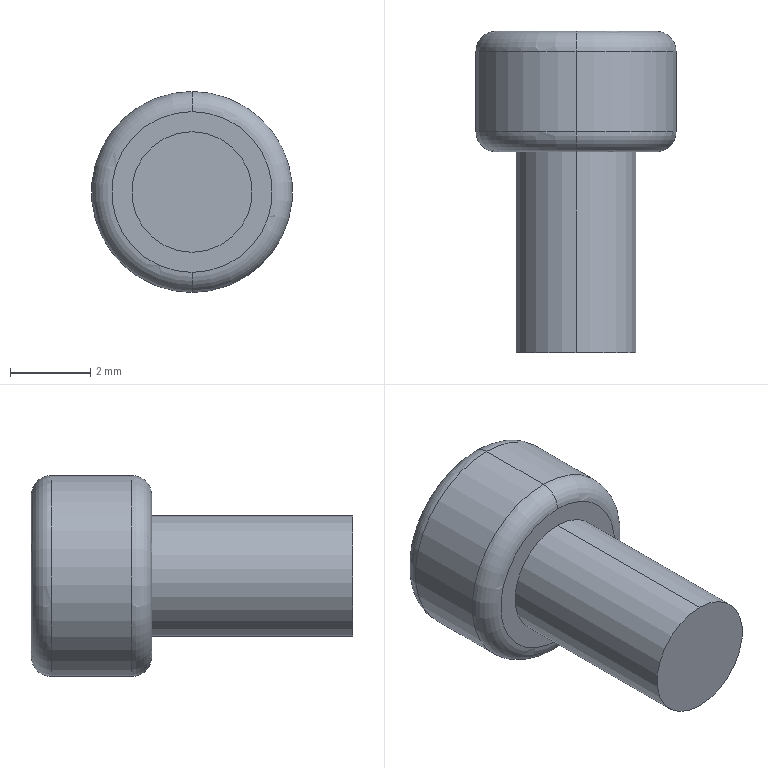Part | NX | features BREP 1 | 1 solid | 18 faces | box 5 x 8 x 5 mm | volume 87.225 mm3 | plane 10 | torus 4 | cylinder 4 | commonest cylinder face diameters 3 x2 5 x2
STEP:
#1=CARTESIAN_POINT('',(0.,2.5,-2.5));
#2=VERTEX_POINT('',#1);
#3=CARTESIAN_POINT('',(0.,2.5,2.5));
#4=VERTEX_POINT('',#3);
#5=CARTESIAN_POINT('',(0.,2.5,0.));
#6=DIRECTION('',(0.,-1.,0.));
#7=DIRECTION('',(0.,0.,1.));
#8=AXIS2_PLACEMENT_3D('',#5,#6,#7);
#9=CIRCLE('',#8,2.5);
#10=EDGE_CURVE('',#2,#4,#9,.T.);
#11=ORIENTED_EDGE('',*,*,#10,.F.);
#12=CARTESIAN_POINT('',(0.,3.,-2.));
#13=VERTEX_POINT('',#12);
#14=CARTESIAN_POINT('',(0.,2.5,-2.));
#15=DIRECTION('',(1.,0.,0.));
#16=DIRECTION('',(0.,0.,-1.));
#17=AXIS2_PLACEMENT_3D('',#14,#15,#16);
#18=CIRCLE('',#17,0.5);
#19=EDGE_CURVE('',#2,#13,#18,.T.);
#20=ORIENTED_EDGE('',*,*,#19,.T.);
#21=CARTESIAN_POINT('',(0.,3.,2.));
#22=VERTEX_POINT('',#21);
#23=CARTESIAN_POINT('',(0.,3.,0.));
#24=DIRECTION('',(0.,1.,0.));
#25=DIRECTION('',(0.,0.,1.));
#26=AXIS2_PLACEMENT_3D('',#23,#24,#25);
#27=CIRCLE('',#26,2.);
#28=EDGE_CURVE('',#22,#13,#27,.T.);
#29=ORIENTED_EDGE('',*,*,#28,.F.);
#30=CARTESIAN_POINT('',(0.,2.5,2.));
#31=DIRECTION('',(-1.,0.,0.));
#32=DIRECTION('',(0.,0.,1.));
#33=AXIS2_PLACEMENT_3D('',#30,#31,#32);
#34=CIRCLE('',#33,0.5);
#35=EDGE_CURVE('',#4,#22,#34,.T.);
#36=ORIENTED_EDGE('',*,*,#35,.F.);
#37=EDGE_LOOP('',(#11,#20,#29,#36));
#38=FACE_BOUND('',#37,.T.);
#39=CARTESIAN_POINT('',(0.,2.5,0.));
#40=DIRECTION('',(0.,1.,0.));
#41=DIRECTION('',(0.,0.,-1.));
#42=AXIS2_PLACEMENT_3D('',#39,#40,#41);
#43=TOROIDAL_SURFACE('',#42,2.,0.5);
#44=ADVANCED_FACE('',(#38),#43,.T.);
#45=CARTESIAN_POINT('',(0.,0.,-2.));
#46=VERTEX_POINT('',#45);
#47=CARTESIAN_POINT('',(0.,0.,2.));
#48=VERTEX_POINT('',#47);
#49=CARTESIAN_POINT('',(0.,0.,0.));
#50=DIRECTION('',(0.,-1.,0.));
#51=DIRECTION('',(0.,0.,1.));
#52=AXIS2_PLACEMENT_3D('',#49,#50,#51);
#53=CIRCLE('',#52,2.);
#54=EDGE_CURVE('',#46,#48,#53,.T.);
#55=ORIENTED_EDGE('',*,*,#54,.F.);
#56=CARTESIAN_POINT('',(0.,0.5,-2.5));
#57=VERTEX_POINT('',#56);
#58=CARTESIAN_POINT('',(0.,0.5,-2.));
#59=DIRECTION('',(1.,0.,0.));
#60=DIRECTION('',(0.,0.,-1.));
#61=AXIS2_PLACEMENT_3D('',#58,#59,#60);
#62=CIRCLE('',#61,0.5);
#63=EDGE_CURVE('',#46,#57,#62,.T.);
#64=ORIENTED_EDGE('',*,*,#63,.T.);
#65=CARTESIAN_POINT('',(0.,0.5,2.5));
#66=VERTEX_POINT('',#65);
#67=CARTESIAN_POINT('',(0.,0.5,0.));
#68=DIRECTION('',(0.,1.,0.));
#69=DIRECTION('',(0.,0.,1.));
#70=AXIS2_PLACEMENT_3D('',#67,#68,#69);
#71=CIRCLE('',#70,2.5);
#72=EDGE_CURVE('',#66,#57,#71,.T.);
#73=ORIENTED_EDGE('',*,*,#72,.F.);
#74=CARTESIAN_POINT('',(0.,0.5,2.));
#75=DIRECTION('',(-1.,0.,0.));
#76=DIRECTION('',(0.,0.,1.));
#77=AXIS2_PLACEMENT_3D('',#74,#75,#76);
#78=CIRCLE('',#77,0.5);
#79=EDGE_CURVE('',#48,#66,#78,.T.);
#80=ORIENTED_EDGE('',*,*,#79,.F.);
#81=EDGE_LOOP('',(#55,#64,#73,#80));
#82=FACE_BOUND('',#81,.T.);
#83=CARTESIAN_POINT('',(0.,0.5,0.));
#84=DIRECTION('',(0.,1.,0.));
#85=DIRECTION('',(0.,0.,-1.));
#86=AXIS2_PLACEMENT_3D('',#83,#84,#85);
#87=TOROIDAL_SURFACE('',#86,2.,0.5);
#88=ADVANCED_FACE('',(#82),#87,.T.);
#89=CARTESIAN_POINT('',(0.,-5.,-1.5));
#90=VERTEX_POINT('',#89);
#91=CARTESIAN_POINT('',(0.,-5.,1.5));
#92=VERTEX_POINT('',#91);
#93=CARTESIAN_POINT('',(0.,-5.,0.));
#94=DIRECTION('',(0.,-1.,0.));
#95=DIRECTION('',(0.,0.,-1.));
#96=AXIS2_PLACEMENT_3D('',#93,#94,#95);
#97=CIRCLE('',#96,1.5);
#98=EDGE_CURVE('',#90,#92,#97,.T.);
#99=ORIENTED_EDGE('',*,*,#98,.F.);
#100=CARTESIAN_POINT('',(0.,0.,-1.5));
#101=VERTEX_POINT('',#100);
#102=CARTESIAN_POINT('',(0.,-5.,-1.5));
#103=DIRECTION('',(0.,1.,0.));
#104=VECTOR('',#103,1000.);
#105=LINE('',#102,#104);
#106=EDGE_CURVE('',#90,#101,#105,.T.);
#107=ORIENTED_EDGE('',*,*,#106,.T.);
#108=CARTESIAN_POINT('',(0.,0.,1.5));
#109=VERTEX_POINT('',#108);
#110=CARTESIAN_POINT('',(0.,0.,0.));
#111=DIRECTION('',(0.,-1.,0.));
#112=DIRECTION('',(0.,0.,-1.));
#113=AXIS2_PLACEMENT_3D('',#110,#111,#112);
#114=CIRCLE('',#113,1.5);
#115=EDGE_CURVE('',#101,#109,#114,.T.);
#116=ORIENTED_EDGE('',*,*,#115,.T.);
#117=CARTESIAN_POINT('',(0.,-5.,1.5));
#118=DIRECTION('',(0.,1.,0.));
#119=VECTOR('',#118,1000.);
#120=LINE('',#117,#119);
#121=EDGE_CURVE('',#92,#109,#120,.T.);
#122=ORIENTED_EDGE('',*,*,#121,.F.);
#123=EDGE_LOOP('',(#99,#107,#116,#122));
#124=FACE_BOUND('',#123,.T.);
#125=CARTESIAN_POINT('',(0.,-5.,0.));
#126=DIRECTION('',(0.,1.,0.));
#127=DIRECTION('',(0.,0.,-1.));
#128=AXIS2_PLACEMENT_3D('',#125,#126,#127);
#129=CYLINDRICAL_SURFACE('',#128,1.5);
#130=ADVANCED_FACE('',(#124),#129,.T.);
#131=ORIENTED_EDGE('',*,*,#10,.T.);
#132=CARTESIAN_POINT('',(0.,3.,2.5));
#133=DIRECTION('',(0.,-1.,0.));
#134=VECTOR('',#133,1000.);
#135=LINE('',#132,#134);
#136=EDGE_CURVE('',#66,#4,#135,.F.);
#137=ORIENTED_EDGE('',*,*,#136,.F.);
#138=ORIENTED_EDGE('',*,*,#72,.T.);
#139=CARTESIAN_POINT('',(0.,3.,-2.5));
#140=DIRECTION('',(0.,-1.,0.));
#141=VECTOR('',#140,1000.);
#142=LINE('',#139,#141);
#143=EDGE_CURVE('',#57,#2,#142,.F.);
#144=ORIENTED_EDGE('',*,*,#143,.T.);
#145=EDGE_LOOP('',(#131,#137,#138,#144));
#146=FACE_BOUND('',#145,.T.);
#147=CARTESIAN_POINT('',(0.,3.,0.));
#148=DIRECTION('',(0.,-1.,0.));
#149=DIRECTION('',(0.,0.,1.));
#150=AXIS2_PLACEMENT_3D('',#147,#148,#149);
#151=CYLINDRICAL_SURFACE('',#150,2.5);
#152=ADVANCED_FACE('',(#146),#151,.T.);
#153=ORIENTED_EDGE('',*,*,#136,.T.);
#154=CARTESIAN_POINT('',(0.,2.5,0.));
#155=DIRECTION('',(0.,-1.,0.));
#156=DIRECTION('',(0.,0.,1.));
#157=AXIS2_PLACEMENT_3D('',#154,#155,#156);
#158=CIRCLE('',#157,2.5);
#159=EDGE_CURVE('',#4,#2,#158,.T.);
#160=ORIENTED_EDGE('',*,*,#159,.T.);
#161=ORIENTED_EDGE('',*,*,#143,.F.);
#162=CARTESIAN_POINT('',(0.,0.5,0.));
#163=DIRECTION('',(0.,1.,0.));
#164=DIRECTION('',(0.,0.,1.));
#165=AXIS2_PLACEMENT_3D('',#162,#163,#164);
#166=CIRCLE('',#165,2.5);
#167=EDGE_CURVE('',#57,#66,#166,.T.);
#168=ORIENTED_EDGE('',*,*,#167,.T.);
#169=EDGE_LOOP('',(#153,#160,#161,#168));
#170=FACE_BOUND('',#169,.T.);
#171=CARTESIAN_POINT('',(0.,3.,0.));
#172=DIRECTION('',(0.,-1.,0.));
#173=DIRECTION('',(0.,0.,1.));
#174=AXIS2_PLACEMENT_3D('',#171,#172,#173);
#175=CYLINDRICAL_SURFACE('',#174,2.5);
#176=ADVANCED_FACE('',(#170),#175,.T.);
#177=ORIENTED_EDGE('',*,*,#28,.T.);
#178=CARTESIAN_POINT('',(0.,3.,0.));
#179=DIRECTION('',(0.,1.,0.));
#180=DIRECTION('',(0.,0.,1.));
#181=AXIS2_PLACEMENT_3D('',#178,#179,#180);
#182=CIRCLE('',#181,2.);
#183=EDGE_CURVE('',#13,#22,#182,.T.);
#184=ORIENTED_EDGE('',*,*,#183,.T.);
#185=EDGE_LOOP('',(#177,#184));
#186=FACE_BOUND('',#185,.T.);
#187=CARTESIAN_POINT('',(0.7217,3.,1.25));
#188=VERTEX_POINT('',#187);
#189=CARTESIAN_POINT('',(1.443,3.,0.));
#190=VERTEX_POINT('',#189);
#191=CARTESIAN_POINT('',(0.7217,3.,1.25));
#192=DIRECTION('',(0.5,0.,-0.866));
#193=VECTOR('',#192,1000.);
#194=LINE('',#191,#193);
#195=EDGE_CURVE('',#188,#190,#194,.T.);
#196=ORIENTED_EDGE('',*,*,#195,.F.);
#197=CARTESIAN_POINT('',(-0.7217,3.,1.25));
#198=VERTEX_POINT('',#197);
#199=CARTESIAN_POINT('',(-0.7217,3.,1.25));
#200=DIRECTION('',(1.,0.,0.));
#201=VECTOR('',#200,1000.);
#202=LINE('',#199,#201);
#203=EDGE_CURVE('',#198,#188,#202,.T.);
#204=ORIENTED_EDGE('',*,*,#203,.F.);
#205=CARTESIAN_POINT('',(-1.443,3.,0.));
#206=VERTEX_POINT('',#205);
#207=CARTESIAN_POINT('',(-1.443,3.,0.));
#208=DIRECTION('',(0.5,0.,0.866));
#209=VECTOR('',#208,1000.);
#210=LINE('',#207,#209);
#211=EDGE_CURVE('',#206,#198,#210,.T.);
#212=ORIENTED_EDGE('',*,*,#211,.F.);
#213=CARTESIAN_POINT('',(-0.7217,3.,-1.25));
#214=VERTEX_POINT('',#213);
#215=CARTESIAN_POINT('',(-0.7217,3.,-1.25));
#216=DIRECTION('',(-0.5,0.,0.866));
#217=VECTOR('',#216,1000.);
#218=LINE('',#215,#217);
#219=EDGE_CURVE('',#214,#206,#218,.T.);
#220=ORIENTED_EDGE('',*,*,#219,.F.);
#221=CARTESIAN_POINT('',(0.7217,3.,-1.25));
#222=VERTEX_POINT('',#221);
#223=CARTESIAN_POINT('',(0.7217,3.,-1.25));
#224=DIRECTION('',(-1.,0.,0.));
#225=VECTOR('',#224,1000.);
#226=LINE('',#223,#225);
#227=EDGE_CURVE('',#222,#214,#226,.T.);
#228=ORIENTED_EDGE('',*,*,#227,.F.);
#229=CARTESIAN_POINT('',(1.443,3.,0.));
#230=DIRECTION('',(-0.5,0.,-0.866));
#231=VECTOR('',#230,1000.);
#232=LINE('',#229,#231);
#233=EDGE_CURVE('',#190,#222,#232,.T.);
#234=ORIENTED_EDGE('',*,*,#233,.F.);
#235=EDGE_LOOP('',(#196,#204,#212,#220,#228,#234));
#236=FACE_BOUND('',#235,.T.);
#237=CARTESIAN_POINT('',(0.,3.,0.));
#238=DIRECTION('',(0.,1.,0.));
#239=DIRECTION('',(-1.,0.,0.));
#240=AXIS2_PLACEMENT_3D('',#237,#238,#239);
#241=PLANE('',#240);
#242=ADVANCED_FACE('',(#186,#236),#241,.T.);
#243=CARTESIAN_POINT('',(0.,0.,0.));
#244=DIRECTION('',(0.,-1.,0.));
#245=DIRECTION('',(0.,0.,1.));
#246=AXIS2_PLACEMENT_3D('',#243,#244,#245);
#247=CIRCLE('',#246,2.);
#248=EDGE_CURVE('',#48,#46,#247,.T.);
#249=ORIENTED_EDGE('',*,*,#248,.T.);
#250=ORIENTED_EDGE('',*,*,#54,.T.);
#251=EDGE_LOOP('',(#249,#250));
#252=FACE_BOUND('',#251,.T.);
#253=CARTESIAN_POINT('',(0.,0.,0.));
#254=DIRECTION('',(0.,-1.,0.));
#255=DIRECTION('',(0.,0.,-1.));
#256=AXIS2_PLACEMENT_3D('',#253,#254,#255);
#257=CIRCLE('',#256,1.5);
#258=EDGE_CURVE('',#109,#101,#257,.T.);
#259=ORIENTED_EDGE('',*,*,#258,.F.);
#260=ORIENTED_EDGE('',*,*,#115,.F.);
#261=EDGE_LOOP('',(#259,#260));
#262=FACE_BOUND('',#261,.T.);
#263=CARTESIAN_POINT('',(0.,0.,0.));
#264=DIRECTION('',(0.,1.,0.));
#265=DIRECTION('',(-1.,0.,0.));
#266=AXIS2_PLACEMENT_3D('',#263,#264,#265);
#267=PLANE('',#266);
#268=ADVANCED_FACE('',(#252,#262),#267,.F.);
#269=ORIENTED_EDGE('',*,*,#195,.T.);
#270=CARTESIAN_POINT('',(1.443,2.,0.));
#271=VERTEX_POINT('',#270);
#272=CARTESIAN_POINT('',(1.443,2.,0.));
#273=DIRECTION('',(0.,1.,0.));
#274=VECTOR('',#273,1000.);
#275=LINE('',#272,#274);
#276=EDGE_CURVE('',#271,#190,#275,.T.);
#277=ORIENTED_EDGE('',*,*,#276,.F.);
#278=CARTESIAN_POINT('',(0.7217,2.,1.25));
#279=VERTEX_POINT('',#278);
#280=CARTESIAN_POINT('',(0.7217,2.,1.25));
#281=DIRECTION('',(0.5,0.,-0.866));
#282=VECTOR('',#281,1000.);
#283=LINE('',#280,#282);
#284=EDGE_CURVE('',#279,#271,#283,.T.);
#285=ORIENTED_EDGE('',*,*,#284,.F.);
#286=CARTESIAN_POINT('',(0.7217,2.,1.25));
#287=DIRECTION('',(0.,1.,0.));
#288=VECTOR('',#287,1000.);
#289=LINE('',#286,#288);
#290=EDGE_CURVE('',#279,#188,#289,.T.);
#291=ORIENTED_EDGE('',*,*,#290,.T.);
#292=EDGE_LOOP('',(#269,#277,#285,#291));
#293=FACE_BOUND('',#292,.T.);
#294=CARTESIAN_POINT('',(0.7217,2.,1.25));
#295=DIRECTION('',(0.866,0.,0.5));
#296=DIRECTION('',(0.,1.,0.));
#297=AXIS2_PLACEMENT_3D('',#294,#295,#296);
#298=PLANE('',#297);
#299=ADVANCED_FACE('',(#293),#298,.F.);
#300=ORIENTED_EDGE('',*,*,#203,.T.);
#301=ORIENTED_EDGE('',*,*,#290,.F.);
#302=CARTESIAN_POINT('',(-0.7217,2.,1.25));
#303=VERTEX_POINT('',#302);
#304=CARTESIAN_POINT('',(-0.7217,2.,1.25));
#305=DIRECTION('',(1.,0.,0.));
#306=VECTOR('',#305,1000.);
#307=LINE('',#304,#306);
#308=EDGE_CURVE('',#303,#279,#307,.T.);
#309=ORIENTED_EDGE('',*,*,#308,.F.);
#310=CARTESIAN_POINT('',(-0.7217,2.,1.25));
#311=DIRECTION('',(0.,1.,0.));
#312=VECTOR('',#311,1000.);
#313=LINE('',#310,#312);
#314=EDGE_CURVE('',#303,#198,#313,.T.);
#315=ORIENTED_EDGE('',*,*,#314,.T.);
#316=EDGE_LOOP('',(#300,#301,#309,#315));
#317=FACE_BOUND('',#316,.T.);
#318=CARTESIAN_POINT('',(-0.7217,2.,1.25));
#319=DIRECTION('',(0.,0.,1.));
#320=DIRECTION('',(-1.,0.,0.));
#321=AXIS2_PLACEMENT_3D('',#318,#319,#320);
#322=PLANE('',#321);
#323=ADVANCED_FACE('',(#317),#322,.F.);
#324=ORIENTED_EDGE('',*,*,#211,.T.);
#325=ORIENTED_EDGE('',*,*,#314,.F.);
#326=CARTESIAN_POINT('',(-1.443,2.,0.));
#327=VERTEX_POINT('',#326);
#328=CARTESIAN_POINT('',(-1.443,2.,0.));
#329=DIRECTION('',(0.5,0.,0.866));
#330=VECTOR('',#329,1000.);
#331=LINE('',#328,#330);
#332=EDGE_CURVE('',#327,#303,#331,.T.);
#333=ORIENTED_EDGE('',*,*,#332,.F.);
#334=CARTESIAN_POINT('',(-1.443,2.,0.));
#335=DIRECTION('',(0.,1.,0.));
#336=VECTOR('',#335,1000.);
#337=LINE('',#334,#336);
#338=EDGE_CURVE('',#327,#206,#337,.T.);
#339=ORIENTED_EDGE('',*,*,#338,.T.);
#340=EDGE_LOOP('',(#324,#325,#333,#339));
#341=FACE_BOUND('',#340,.T.);
#342=CARTESIAN_POINT('',(-1.443,2.,0.));
#343=DIRECTION('',(-0.866,0.,0.5));
#344=DIRECTION('',(0.,-1.,0.));
#345=AXIS2_PLACEMENT_3D('',#342,#343,#344);
#346=PLANE('',#345);
#347=ADVANCED_FACE('',(#341),#346,.F.);
#348=ORIENTED_EDGE('',*,*,#219,.T.);
#349=ORIENTED_EDGE('',*,*,#338,.F.);
#350=CARTESIAN_POINT('',(-0.7217,2.,-1.25));
#351=VERTEX_POINT('',#350);
#352=CARTESIAN_POINT('',(-0.7217,2.,-1.25));
#353=DIRECTION('',(-0.5,0.,0.866));
#354=VECTOR('',#353,1000.);
#355=LINE('',#352,#354);
#356=EDGE_CURVE('',#351,#327,#355,.T.);
#357=ORIENTED_EDGE('',*,*,#356,.F.);
#358=CARTESIAN_POINT('',(-0.7217,2.,-1.25));
#359=DIRECTION('',(0.,1.,0.));
#360=VECTOR('',#359,1000.);
#361=LINE('',#358,#360);
#362=EDGE_CURVE('',#351,#214,#361,.T.);
#363=ORIENTED_EDGE('',*,*,#362,.T.);
#364=EDGE_LOOP('',(#348,#349,#357,#363));
#365=FACE_BOUND('',#364,.T.);
#366=CARTESIAN_POINT('',(-0.7217,2.,-1.25));
#367=DIRECTION('',(-0.866,0.,-0.5));
#368=DIRECTION('',(0.5,0.,-0.866));
#369=AXIS2_PLACEMENT_3D('',#366,#367,#368);
#370=PLANE('',#369);
#371=ADVANCED_FACE('',(#365),#370,.F.);
#372=ORIENTED_EDGE('',*,*,#227,.T.);
#373=ORIENTED_EDGE('',*,*,#362,.F.);
#374=CARTESIAN_POINT('',(0.7217,2.,-1.25));
#375=VERTEX_POINT('',#374);
#376=CARTESIAN_POINT('',(0.7217,2.,-1.25));
#377=DIRECTION('',(-1.,0.,0.));
#378=VECTOR('',#377,1000.);
#379=LINE('',#376,#378);
#380=EDGE_CURVE('',#375,#351,#379,.T.);
#381=ORIENTED_EDGE('',*,*,#380,.F.);
#382=CARTESIAN_POINT('',(0.7217,2.,-1.25));
#383=DIRECTION('',(0.,1.,0.));
#384=VECTOR('',#383,1000.);
#385=LINE('',#382,#384);
#386=EDGE_CURVE('',#375,#222,#385,.T.);
#387=ORIENTED_EDGE('',*,*,#386,.T.);
#388=EDGE_LOOP('',(#372,#373,#381,#387));
#389=FACE_BOUND('',#388,.T.);
#390=CARTESIAN_POINT('',(0.7217,2.,-1.25));
#391=DIRECTION('',(0.,0.,-1.));
#392=DIRECTION('',(0.,1.,0.));
#393=AXIS2_PLACEMENT_3D('',#390,#391,#392);
#394=PLANE('',#393);
#395=ADVANCED_FACE('',(#389),#394,.F.);
#396=ORIENTED_EDGE('',*,*,#233,.T.);
#397=ORIENTED_EDGE('',*,*,#386,.F.);
#398=CARTESIAN_POINT('',(1.443,2.,0.));
#399=DIRECTION('',(-0.5,0.,-0.866));
#400=VECTOR('',#399,1000.);
#401=LINE('',#398,#400);
#402=EDGE_CURVE('',#271,#375,#401,.T.);
#403=ORIENTED_EDGE('',*,*,#402,.F.);
#404=ORIENTED_EDGE('',*,*,#276,.T.);
#405=EDGE_LOOP('',(#396,#397,#403,#404));
#406=FACE_BOUND('',#405,.T.);
#407=CARTESIAN_POINT('',(1.443,2.,0.));
#408=DIRECTION('',(0.866,0.,-0.5));
#409=DIRECTION('',(0.,1.,0.));
#410=AXIS2_PLACEMENT_3D('',#407,#408,#409);
#411=PLANE('',#410);
#412=ADVANCED_FACE('',(#406),#411,.F.);
#413=ORIENTED_EDGE('',*,*,#284,.T.);
#414=ORIENTED_EDGE('',*,*,#402,.T.);
#415=ORIENTED_EDGE('',*,*,#380,.T.);
#416=ORIENTED_EDGE('',*,*,#356,.T.);
#417=ORIENTED_EDGE('',*,*,#332,.T.);
#418=ORIENTED_EDGE('',*,*,#308,.T.);
#419=EDGE_LOOP('',(#413,#414,#415,#416,#417,#418));
#420=FACE_BOUND('',#419,.T.);
#421=CARTESIAN_POINT('',(0.,2.,0.));
#422=DIRECTION('',(0.,1.,0.));
#423=DIRECTION('',(-1.,0.,0.));
#424=AXIS2_PLACEMENT_3D('',#421,#422,#423);
#425=PLANE('',#424);
#426=ADVANCED_FACE('',(#420),#425,.T.);
#427=ORIENTED_EDGE('',*,*,#106,.F.);
#428=CARTESIAN_POINT('',(0.,-5.,0.));
#429=DIRECTION('',(0.,-1.,0.));
#430=DIRECTION('',(0.,0.,-1.));
#431=AXIS2_PLACEMENT_3D('',#428,#429,#430);
#432=CIRCLE('',#431,1.5);
#433=EDGE_CURVE('',#92,#90,#432,.T.);
#434=ORIENTED_EDGE('',*,*,#433,.F.);
#435=ORIENTED_EDGE('',*,*,#121,.T.);
#436=ORIENTED_EDGE('',*,*,#258,.T.);
#437=EDGE_LOOP('',(#427,#434,#435,#436));
#438=FACE_BOUND('',#437,.T.);
#439=CARTESIAN_POINT('',(0.,-5.,0.));
#440=DIRECTION('',(0.,1.,0.));
#441=DIRECTION('',(0.,0.,-1.));
#442=AXIS2_PLACEMENT_3D('',#439,#440,#441);
#443=CYLINDRICAL_SURFACE('',#442,1.5);
#444=ADVANCED_FACE('',(#438),#443,.T.);
#445=ORIENTED_EDGE('',*,*,#433,.T.);
#446=ORIENTED_EDGE('',*,*,#98,.T.);
#447=EDGE_LOOP('',(#445,#446));
#448=FACE_BOUND('',#447,.T.);
#449=CARTESIAN_POINT('',(0.,-5.,0.));
#450=DIRECTION('',(0.,-1.,0.));
#451=DIRECTION('',(0.,0.,1.));
#452=AXIS2_PLACEMENT_3D('',#449,#450,#451);
#453=PLANE('',#452);
#454=ADVANCED_FACE('',(#448),#453,.T.);
#455=ORIENTED_EDGE('',*,*,#63,.F.);
#456=ORIENTED_EDGE('',*,*,#248,.F.);
#457=ORIENTED_EDGE('',*,*,#79,.T.);
#458=ORIENTED_EDGE('',*,*,#167,.F.);
#459=EDGE_LOOP('',(#455,#456,#457,#458));
#460=FACE_BOUND('',#459,.T.);
#461=CARTESIAN_POINT('',(0.,0.5,0.));
#462=DIRECTION('',(0.,1.,0.));
#463=DIRECTION('',(0.,0.,-1.));
#464=AXIS2_PLACEMENT_3D('',#461,#462,#463);
#465=TOROIDAL_SURFACE('',#464,2.,0.5);
#466=ADVANCED_FACE('',(#460),#465,.T.);
#467=ORIENTED_EDGE('',*,*,#19,.F.);
#468=ORIENTED_EDGE('',*,*,#159,.F.);
#469=ORIENTED_EDGE('',*,*,#35,.T.);
#470=ORIENTED_EDGE('',*,*,#183,.F.);
#471=EDGE_LOOP('',(#467,#468,#469,#470));
#472=FACE_BOUND('',#471,.T.);
#473=CARTESIAN_POINT('',(0.,2.5,0.));
#474=DIRECTION('',(0.,1.,0.));
#475=DIRECTION('',(0.,0.,-1.));
#476=AXIS2_PLACEMENT_3D('',#473,#474,#475);
#477=TOROIDAL_SURFACE('',#476,2.,0.5);
#478=ADVANCED_FACE('',(#472),#477,.T.);
#479=CLOSED_SHELL('',(#44,#88,#130,#152,#176,#242,#268,#299,#323,#347,#371,#395,#412,#426,#444,#454,#466,#478));
#480=MANIFOLD_SOLID_BREP('',#479);
#481=(LENGTH_UNIT()NAMED_UNIT(*)SI_UNIT(.MILLI.,.METRE.));
#482=UNCERTAINTY_MEASURE_WITH_UNIT(LENGTH_MEASURE(0.00001),#481,'','');
#483=(NAMED_UNIT(*)PLANE_ANGLE_UNIT()SI_UNIT($,.RADIAN.));
#484=(NAMED_UNIT(*)SI_UNIT($,.STERADIAN.)SOLID_ANGLE_UNIT());
#485=(GEOMETRIC_REPRESENTATION_CONTEXT(3)GLOBAL_UNCERTAINTY_ASSIGNED_CONTEXT((#482))GLOBAL_UNIT_ASSIGNED_CONTEXT((#481,#483,#484))REPRESENTATION_CONTEXT('',''));
#486=ADVANCED_BREP_SHAPE_REPRESENTATION('',(#480),#485);